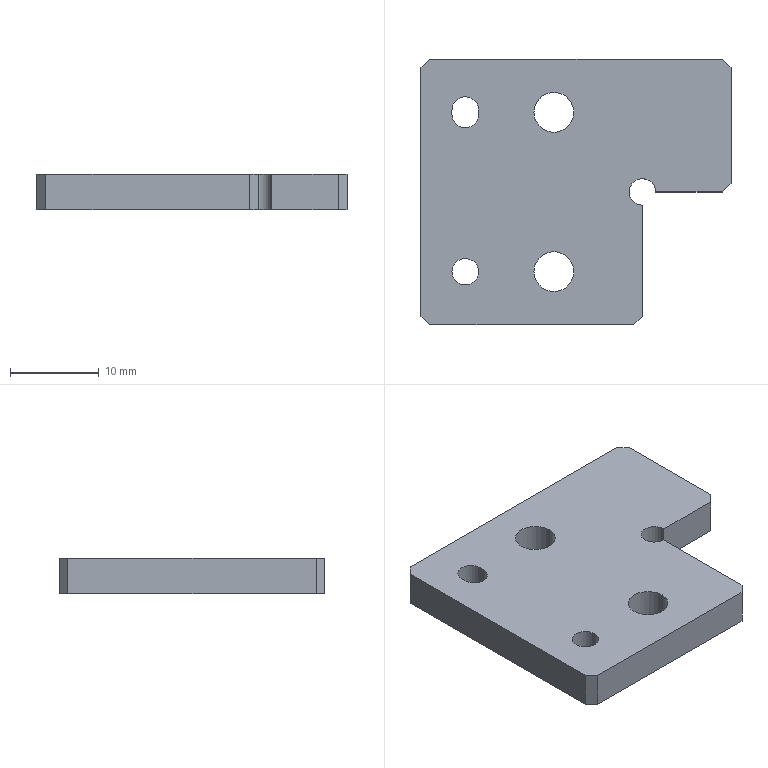Part | SolidWorks | features HoleWzd 3, ICE 2, Chamfer 1, Extrusion 1 | 1 solid | 24 faces | box 35 x 30 x 4 mm | volume 3379 mm3 | plane 15 | cylinder 9 | commonest cylinder face diameters 3 x5 4.5 x4
STEP:
#1=CARTESIAN_POINT('',(-4.75,9.,-2.));
#2=VERTEX_POINT('',#1);
#3=CARTESIAN_POINT('',(-0.25,9.,-2.));
#4=VERTEX_POINT('',#3);
#5=CARTESIAN_POINT('',(-2.5,9.,-2.));
#6=DIRECTION('',(0.,0.,1.));
#7=DIRECTION('',(1.,0.,0.));
#8=AXIS2_PLACEMENT_3D('',#5,#6,#7);
#9=CIRCLE('',#8,2.25);
#10=EDGE_CURVE('',#2,#4,#9,.T.);
#11=ORIENTED_EDGE('',*,*,#10,.F.);
#12=CARTESIAN_POINT('',(-4.75,9.,2.));
#13=VERTEX_POINT('',#12);
#14=CARTESIAN_POINT('',(-4.75,9.,2.));
#15=DIRECTION('',(0.,0.,1.));
#16=VECTOR('',#15,1000.);
#17=LINE('',#14,#16);
#18=EDGE_CURVE('',#2,#13,#17,.T.);
#19=ORIENTED_EDGE('',*,*,#18,.T.);
#20=CARTESIAN_POINT('',(-0.25,9.,2.));
#21=VERTEX_POINT('',#20);
#22=CARTESIAN_POINT('',(-2.5,9.,2.));
#23=DIRECTION('',(0.,0.,1.));
#24=DIRECTION('',(1.,0.,0.));
#25=AXIS2_PLACEMENT_3D('',#22,#23,#24);
#26=CIRCLE('',#25,2.25);
#27=EDGE_CURVE('',#13,#21,#26,.T.);
#28=ORIENTED_EDGE('',*,*,#27,.T.);
#29=CARTESIAN_POINT('',(-0.25,9.,2.));
#30=DIRECTION('',(0.,0.,1.));
#31=VECTOR('',#30,1000.);
#32=LINE('',#29,#31);
#33=EDGE_CURVE('',#4,#21,#32,.T.);
#34=ORIENTED_EDGE('',*,*,#33,.F.);
#35=EDGE_LOOP('',(#11,#19,#28,#34));
#36=FACE_OUTER_BOUND('',#35,.T.);
#37=CARTESIAN_POINT('',(-2.5,9.,2.));
#38=DIRECTION('',(0.,0.,1.));
#39=DIRECTION('',(1.,0.,0.));
#40=AXIS2_PLACEMENT_3D('',#37,#38,#39);
#41=CYLINDRICAL_SURFACE('',#40,2.25);
#42=ADVANCED_FACE('',(#36),#41,.F.);
#43=CARTESIAN_POINT('',(-4.75,-9.,-2.));
#44=VERTEX_POINT('',#43);
#45=CARTESIAN_POINT('',(-0.25,-9.,-2.));
#46=VERTEX_POINT('',#45);
#47=CARTESIAN_POINT('',(-2.5,-9.,-2.));
#48=DIRECTION('',(0.,0.,1.));
#49=DIRECTION('',(1.,0.,0.));
#50=AXIS2_PLACEMENT_3D('',#47,#48,#49);
#51=CIRCLE('',#50,2.25);
#52=EDGE_CURVE('',#44,#46,#51,.T.);
#53=ORIENTED_EDGE('',*,*,#52,.F.);
#54=CARTESIAN_POINT('',(-4.75,-9.,2.));
#55=VERTEX_POINT('',#54);
#56=CARTESIAN_POINT('',(-4.75,-9.,2.));
#57=DIRECTION('',(0.,0.,1.));
#58=VECTOR('',#57,1000.);
#59=LINE('',#56,#58);
#60=EDGE_CURVE('',#44,#55,#59,.T.);
#61=ORIENTED_EDGE('',*,*,#60,.T.);
#62=CARTESIAN_POINT('',(-0.25,-9.,2.));
#63=VERTEX_POINT('',#62);
#64=CARTESIAN_POINT('',(-2.5,-9.,2.));
#65=DIRECTION('',(0.,0.,1.));
#66=DIRECTION('',(1.,0.,0.));
#67=AXIS2_PLACEMENT_3D('',#64,#65,#66);
#68=CIRCLE('',#67,2.25);
#69=EDGE_CURVE('',#55,#63,#68,.T.);
#70=ORIENTED_EDGE('',*,*,#69,.T.);
#71=CARTESIAN_POINT('',(-0.25,-9.,2.));
#72=DIRECTION('',(0.,0.,1.));
#73=VECTOR('',#72,1000.);
#74=LINE('',#71,#73);
#75=EDGE_CURVE('',#46,#63,#74,.T.);
#76=ORIENTED_EDGE('',*,*,#75,.F.);
#77=EDGE_LOOP('',(#53,#61,#70,#76));
#78=FACE_OUTER_BOUND('',#77,.T.);
#79=CARTESIAN_POINT('',(-2.5,-9.,2.));
#80=DIRECTION('',(0.,0.,1.));
#81=DIRECTION('',(1.,0.,0.));
#82=AXIS2_PLACEMENT_3D('',#79,#80,#81);
#83=CYLINDRICAL_SURFACE('',#82,2.25);
#84=ADVANCED_FACE('',(#78),#83,.F.);
#85=CARTESIAN_POINT('',(-14.,-9.,-2.));
#86=VERTEX_POINT('',#85);
#87=CARTESIAN_POINT('',(-11.,-9.,-2.));
#88=VERTEX_POINT('',#87);
#89=CARTESIAN_POINT('',(-12.5,-9.,-2.));
#90=DIRECTION('',(0.,0.,1.));
#91=DIRECTION('',(1.,0.,0.));
#92=AXIS2_PLACEMENT_3D('',#89,#90,#91);
#93=CIRCLE('',#92,1.5);
#94=EDGE_CURVE('',#86,#88,#93,.T.);
#95=ORIENTED_EDGE('',*,*,#94,.F.);
#96=CARTESIAN_POINT('',(-14.,-9.,2.));
#97=VERTEX_POINT('',#96);
#98=CARTESIAN_POINT('',(-14.,-9.,2.));
#99=DIRECTION('',(0.,0.,1.));
#100=VECTOR('',#99,1000.);
#101=LINE('',#98,#100);
#102=EDGE_CURVE('',#86,#97,#101,.T.);
#103=ORIENTED_EDGE('',*,*,#102,.T.);
#104=CARTESIAN_POINT('',(-11.,-9.,2.));
#105=VERTEX_POINT('',#104);
#106=CARTESIAN_POINT('',(-12.5,-9.,2.));
#107=DIRECTION('',(0.,0.,1.));
#108=DIRECTION('',(1.,0.,0.));
#109=AXIS2_PLACEMENT_3D('',#106,#107,#108);
#110=CIRCLE('',#109,1.5);
#111=EDGE_CURVE('',#97,#105,#110,.T.);
#112=ORIENTED_EDGE('',*,*,#111,.T.);
#113=CARTESIAN_POINT('',(-11.,-9.,2.));
#114=DIRECTION('',(0.,0.,1.));
#115=VECTOR('',#114,1000.);
#116=LINE('',#113,#115);
#117=EDGE_CURVE('',#88,#105,#116,.T.);
#118=ORIENTED_EDGE('',*,*,#117,.F.);
#119=EDGE_LOOP('',(#95,#103,#112,#118));
#120=FACE_OUTER_BOUND('',#119,.T.);
#121=CARTESIAN_POINT('',(-12.5,-9.,2.));
#122=DIRECTION('',(0.,0.,1.));
#123=DIRECTION('',(1.,0.,0.));
#124=AXIS2_PLACEMENT_3D('',#121,#122,#123);
#125=CYLINDRICAL_SURFACE('',#124,1.5);
#126=ADVANCED_FACE('',(#120),#125,.F.);
#127=CARTESIAN_POINT('',(17.5,1.,-2.));
#128=VERTEX_POINT('',#127);
#129=CARTESIAN_POINT('',(17.5,14.,-2.));
#130=VERTEX_POINT('',#129);
#131=CARTESIAN_POINT('',(17.5,15.,-2.));
#132=DIRECTION('',(0.,1.,0.));
#133=VECTOR('',#132,1000.);
#134=LINE('',#131,#133);
#135=EDGE_CURVE('',#128,#130,#134,.T.);
#136=ORIENTED_EDGE('',*,*,#135,.T.);
#137=CARTESIAN_POINT('',(17.5,14.,2.));
#138=VERTEX_POINT('',#137);
#139=CARTESIAN_POINT('',(17.5,14.,2.));
#140=DIRECTION('',(0.,0.,1.));
#141=VECTOR('',#140,1000.);
#142=LINE('',#139,#141);
#143=EDGE_CURVE('',#130,#138,#142,.T.);
#144=ORIENTED_EDGE('',*,*,#143,.T.);
#145=CARTESIAN_POINT('',(17.5,1.,2.));
#146=VERTEX_POINT('',#145);
#147=CARTESIAN_POINT('',(17.5,15.,2.));
#148=DIRECTION('',(0.,1.,0.));
#149=VECTOR('',#148,1000.);
#150=LINE('',#147,#149);
#151=EDGE_CURVE('',#146,#138,#150,.T.);
#152=ORIENTED_EDGE('',*,*,#151,.F.);
#153=CARTESIAN_POINT('',(17.5,1.,2.));
#154=DIRECTION('',(0.,0.,-1.));
#155=VECTOR('',#154,1000.);
#156=LINE('',#153,#155);
#157=EDGE_CURVE('',#146,#128,#156,.T.);
#158=ORIENTED_EDGE('',*,*,#157,.T.);
#159=EDGE_LOOP('',(#136,#144,#152,#158));
#160=FACE_OUTER_BOUND('',#159,.T.);
#161=CARTESIAN_POINT('',(17.5,15.,2.));
#162=DIRECTION('',(-1.,0.,0.));
#163=DIRECTION('',(0.,-1.,0.));
#164=AXIS2_PLACEMENT_3D('',#161,#162,#163);
#165=PLANE('',#164);
#166=ADVANCED_FACE('',(#160),#165,.F.);
#167=CARTESIAN_POINT('',(16.5,15.,-2.));
#168=VERTEX_POINT('',#167);
#169=CARTESIAN_POINT('',(-16.5,15.,-2.));
#170=VERTEX_POINT('',#169);
#171=CARTESIAN_POINT('',(-17.5,15.,-2.));
#172=DIRECTION('',(-1.,0.,0.));
#173=VECTOR('',#172,1000.);
#174=LINE('',#171,#173);
#175=EDGE_CURVE('',#168,#170,#174,.T.);
#176=ORIENTED_EDGE('',*,*,#175,.T.);
#177=CARTESIAN_POINT('',(-16.5,15.,2.));
#178=VERTEX_POINT('',#177);
#179=CARTESIAN_POINT('',(-16.5,15.,2.));
#180=DIRECTION('',(0.,0.,1.));
#181=VECTOR('',#180,1000.);
#182=LINE('',#179,#181);
#183=EDGE_CURVE('',#170,#178,#182,.T.);
#184=ORIENTED_EDGE('',*,*,#183,.T.);
#185=CARTESIAN_POINT('',(16.5,15.,2.));
#186=VERTEX_POINT('',#185);
#187=CARTESIAN_POINT('',(-17.5,15.,2.));
#188=DIRECTION('',(-1.,0.,0.));
#189=VECTOR('',#188,1000.);
#190=LINE('',#187,#189);
#191=EDGE_CURVE('',#186,#178,#190,.T.);
#192=ORIENTED_EDGE('',*,*,#191,.F.);
#193=CARTESIAN_POINT('',(16.5,15.,2.));
#194=DIRECTION('',(0.,0.,-1.));
#195=VECTOR('',#194,1000.);
#196=LINE('',#193,#195);
#197=EDGE_CURVE('',#186,#168,#196,.T.);
#198=ORIENTED_EDGE('',*,*,#197,.T.);
#199=EDGE_LOOP('',(#176,#184,#192,#198));
#200=FACE_OUTER_BOUND('',#199,.T.);
#201=CARTESIAN_POINT('',(-17.5,15.,2.));
#202=DIRECTION('',(0.,-1.,0.));
#203=DIRECTION('',(0.,0.,-1.));
#204=AXIS2_PLACEMENT_3D('',#201,#202,#203);
#205=PLANE('',#204);
#206=ADVANCED_FACE('',(#200),#205,.F.);
#207=CARTESIAN_POINT('',(-17.5,14.,2.));
#208=VERTEX_POINT('',#207);
#209=CARTESIAN_POINT('',(-17.5,-14.,2.));
#210=VERTEX_POINT('',#209);
#211=CARTESIAN_POINT('',(-17.5,15.,2.));
#212=DIRECTION('',(0.,-1.,0.));
#213=VECTOR('',#212,1000.);
#214=LINE('',#211,#213);
#215=EDGE_CURVE('',#208,#210,#214,.T.);
#216=ORIENTED_EDGE('',*,*,#215,.F.);
#217=CARTESIAN_POINT('',(-17.5,14.,-2.));
#218=VERTEX_POINT('',#217);
#219=CARTESIAN_POINT('',(-17.5,14.,2.));
#220=DIRECTION('',(0.,0.,-1.));
#221=VECTOR('',#220,1000.);
#222=LINE('',#219,#221);
#223=EDGE_CURVE('',#208,#218,#222,.T.);
#224=ORIENTED_EDGE('',*,*,#223,.T.);
#225=CARTESIAN_POINT('',(-17.5,-14.,-2.));
#226=VERTEX_POINT('',#225);
#227=CARTESIAN_POINT('',(-17.5,15.,-2.));
#228=DIRECTION('',(0.,-1.,0.));
#229=VECTOR('',#228,1000.);
#230=LINE('',#227,#229);
#231=EDGE_CURVE('',#218,#226,#230,.T.);
#232=ORIENTED_EDGE('',*,*,#231,.T.);
#233=CARTESIAN_POINT('',(-17.5,-14.,2.));
#234=DIRECTION('',(0.,0.,1.));
#235=VECTOR('',#234,1000.);
#236=LINE('',#233,#235);
#237=EDGE_CURVE('',#226,#210,#236,.T.);
#238=ORIENTED_EDGE('',*,*,#237,.T.);
#239=EDGE_LOOP('',(#216,#224,#232,#238));
#240=FACE_OUTER_BOUND('',#239,.T.);
#241=CARTESIAN_POINT('',(-17.5,15.,2.));
#242=DIRECTION('',(1.,0.,0.));
#243=DIRECTION('',(0.,0.,-1.));
#244=AXIS2_PLACEMENT_3D('',#241,#242,#243);
#245=PLANE('',#244);
#246=ADVANCED_FACE('',(#240),#245,.F.);
#247=CARTESIAN_POINT('',(-16.5,-15.,-2.));
#248=VERTEX_POINT('',#247);
#249=CARTESIAN_POINT('',(6.5,-15.,-2.));
#250=VERTEX_POINT('',#249);
#251=CARTESIAN_POINT('',(-17.5,-15.,-2.));
#252=DIRECTION('',(1.,0.,0.));
#253=VECTOR('',#252,1000.);
#254=LINE('',#251,#253);
#255=EDGE_CURVE('',#248,#250,#254,.T.);
#256=ORIENTED_EDGE('',*,*,#255,.T.);
#257=CARTESIAN_POINT('',(6.5,-15.,2.));
#258=VERTEX_POINT('',#257);
#259=CARTESIAN_POINT('',(6.5,-15.,2.));
#260=DIRECTION('',(0.,0.,1.));
#261=VECTOR('',#260,1000.);
#262=LINE('',#259,#261);
#263=EDGE_CURVE('',#250,#258,#262,.T.);
#264=ORIENTED_EDGE('',*,*,#263,.T.);
#265=CARTESIAN_POINT('',(-16.5,-15.,2.));
#266=VERTEX_POINT('',#265);
#267=CARTESIAN_POINT('',(-17.5,-15.,2.));
#268=DIRECTION('',(1.,0.,0.));
#269=VECTOR('',#268,1000.);
#270=LINE('',#267,#269);
#271=EDGE_CURVE('',#266,#258,#270,.T.);
#272=ORIENTED_EDGE('',*,*,#271,.F.);
#273=CARTESIAN_POINT('',(-16.5,-15.,2.));
#274=DIRECTION('',(0.,0.,-1.));
#275=VECTOR('',#274,1000.);
#276=LINE('',#273,#275);
#277=EDGE_CURVE('',#266,#248,#276,.T.);
#278=ORIENTED_EDGE('',*,*,#277,.T.);
#279=EDGE_LOOP('',(#256,#264,#272,#278));
#280=FACE_OUTER_BOUND('',#279,.T.);
#281=CARTESIAN_POINT('',(-17.5,-15.,2.));
#282=DIRECTION('',(0.,1.,0.));
#283=DIRECTION('',(0.,0.,1.));
#284=AXIS2_PLACEMENT_3D('',#281,#282,#283);
#285=PLANE('',#284);
#286=ADVANCED_FACE('',(#280),#285,.F.);
#287=CARTESIAN_POINT('',(-11.,9.25,2.));
#288=VERTEX_POINT('',#287);
#289=CARTESIAN_POINT('',(-14.,9.25,2.));
#290=VERTEX_POINT('',#289);
#291=CARTESIAN_POINT('',(-12.5,9.25,2.));
#292=DIRECTION('',(0.,0.,1.));
#293=DIRECTION('',(1.,0.,0.));
#294=AXIS2_PLACEMENT_3D('',#291,#292,#293);
#295=CIRCLE('',#294,1.5);
#296=EDGE_CURVE('',#288,#290,#295,.T.);
#297=ORIENTED_EDGE('',*,*,#296,.F.);
#298=CARTESIAN_POINT('',(-11.,8.75,2.));
#299=VERTEX_POINT('',#298);
#300=CARTESIAN_POINT('',(-11.,9.25,2.));
#301=DIRECTION('',(0.,1.,0.));
#302=VECTOR('',#301,1000.);
#303=LINE('',#300,#302);
#304=EDGE_CURVE('',#299,#288,#303,.T.);
#305=ORIENTED_EDGE('',*,*,#304,.F.);
#306=CARTESIAN_POINT('',(-14.,8.75,2.));
#307=VERTEX_POINT('',#306);
#308=CARTESIAN_POINT('',(-12.5,8.75,2.));
#309=DIRECTION('',(0.,0.,1.));
#310=DIRECTION('',(1.,0.,0.));
#311=AXIS2_PLACEMENT_3D('',#308,#309,#310);
#312=CIRCLE('',#311,1.5);
#313=EDGE_CURVE('',#307,#299,#312,.T.);
#314=ORIENTED_EDGE('',*,*,#313,.F.);
#315=CARTESIAN_POINT('',(-14.,9.25,2.));
#316=DIRECTION('',(0.,-1.,0.));
#317=VECTOR('',#316,1000.);
#318=LINE('',#315,#317);
#319=EDGE_CURVE('',#290,#307,#318,.T.);
#320=ORIENTED_EDGE('',*,*,#319,.F.);
#321=EDGE_LOOP('',(#297,#305,#314,#320));
#322=FACE_BOUND('',#321,.T.);
#323=CARTESIAN_POINT('',(-2.5,9.,2.));
#324=DIRECTION('',(0.,0.,1.));
#325=DIRECTION('',(1.,0.,0.));
#326=AXIS2_PLACEMENT_3D('',#323,#324,#325);
#327=CIRCLE('',#326,2.25);
#328=EDGE_CURVE('',#21,#13,#327,.T.);
#329=ORIENTED_EDGE('',*,*,#328,.F.);
#330=ORIENTED_EDGE('',*,*,#27,.F.);
#331=EDGE_LOOP('',(#329,#330));
#332=FACE_BOUND('',#331,.T.);
#333=CARTESIAN_POINT('',(-2.5,-9.,2.));
#334=DIRECTION('',(0.,0.,1.));
#335=DIRECTION('',(1.,0.,0.));
#336=AXIS2_PLACEMENT_3D('',#333,#334,#335);
#337=CIRCLE('',#336,2.25);
#338=EDGE_CURVE('',#63,#55,#337,.T.);
#339=ORIENTED_EDGE('',*,*,#338,.F.);
#340=ORIENTED_EDGE('',*,*,#69,.F.);
#341=EDGE_LOOP('',(#339,#340));
#342=FACE_BOUND('',#341,.T.);
#343=CARTESIAN_POINT('',(-12.5,-9.,2.));
#344=DIRECTION('',(0.,0.,1.));
#345=DIRECTION('',(1.,0.,0.));
#346=AXIS2_PLACEMENT_3D('',#343,#344,#345);
#347=CIRCLE('',#346,1.5);
#348=EDGE_CURVE('',#105,#97,#347,.T.);
#349=ORIENTED_EDGE('',*,*,#348,.F.);
#350=ORIENTED_EDGE('',*,*,#111,.F.);
#351=EDGE_LOOP('',(#349,#350));
#352=FACE_BOUND('',#351,.T.);
#353=ORIENTED_EDGE('',*,*,#191,.T.);
#354=CARTESIAN_POINT('',(-15.75,15.75,2.));
#355=DIRECTION('',(-0.7071,-0.7071,0.));
#356=VECTOR('',#355,1000.);
#357=LINE('',#354,#356);
#358=EDGE_CURVE('',#178,#208,#357,.T.);
#359=ORIENTED_EDGE('',*,*,#358,.T.);
#360=ORIENTED_EDGE('',*,*,#215,.T.);
#361=CARTESIAN_POINT('',(-15.75,-15.75,2.));
#362=DIRECTION('',(0.7071,-0.7071,0.));
#363=VECTOR('',#362,1000.);
#364=LINE('',#361,#363);
#365=EDGE_CURVE('',#210,#266,#364,.T.);
#366=ORIENTED_EDGE('',*,*,#365,.T.);
#367=ORIENTED_EDGE('',*,*,#271,.T.);
#368=CARTESIAN_POINT('',(7.5,-14.,2.));
#369=VERTEX_POINT('',#368);
#370=CARTESIAN_POINT('',(10.75,-10.75,2.));
#371=DIRECTION('',(0.7071,0.7071,0.));
#372=VECTOR('',#371,1000.);
#373=LINE('',#370,#372);
#374=EDGE_CURVE('',#258,#369,#373,.T.);
#375=ORIENTED_EDGE('',*,*,#374,.T.);
#376=CARTESIAN_POINT('',(7.5,-1.5,2.));
#377=VERTEX_POINT('',#376);
#378=CARTESIAN_POINT('',(7.5,-15.,2.));
#379=DIRECTION('',(0.,-1.,0.));
#380=VECTOR('',#379,1000.);
#381=LINE('',#378,#380);
#382=EDGE_CURVE('',#377,#369,#381,.T.);
#383=ORIENTED_EDGE('',*,*,#382,.F.);
#384=CARTESIAN_POINT('',(9.,0.,2.));
#385=VERTEX_POINT('',#384);
#386=CARTESIAN_POINT('',(7.5,0.,2.));
#387=DIRECTION('',(0.,0.,1.));
#388=DIRECTION('',(1.,0.,0.));
#389=AXIS2_PLACEMENT_3D('',#386,#387,#388);
#390=CIRCLE('',#389,1.5);
#391=EDGE_CURVE('',#385,#377,#390,.T.);
#392=ORIENTED_EDGE('',*,*,#391,.F.);
#393=CARTESIAN_POINT('',(16.5,0.,2.));
#394=VERTEX_POINT('',#393);
#395=CARTESIAN_POINT('',(17.5,0.,2.));
#396=DIRECTION('',(-1.,0.,0.));
#397=VECTOR('',#396,1000.);
#398=LINE('',#395,#397);
#399=EDGE_CURVE('',#394,#385,#398,.T.);
#400=ORIENTED_EDGE('',*,*,#399,.F.);
#401=CARTESIAN_POINT('',(8.25,-8.25,2.));
#402=DIRECTION('',(0.7071,0.7071,0.));
#403=VECTOR('',#402,1000.);
#404=LINE('',#401,#403);
#405=EDGE_CURVE('',#394,#146,#404,.T.);
#406=ORIENTED_EDGE('',*,*,#405,.T.);
#407=ORIENTED_EDGE('',*,*,#151,.T.);
#408=CARTESIAN_POINT('',(15.75,15.75,2.));
#409=DIRECTION('',(-0.7071,0.7071,0.));
#410=VECTOR('',#409,1000.);
#411=LINE('',#408,#410);
#412=EDGE_CURVE('',#138,#186,#411,.T.);
#413=ORIENTED_EDGE('',*,*,#412,.T.);
#414=EDGE_LOOP('',(#353,#359,#360,#366,#367,#375,#383,#392,#400,#406,#407,#413));
#415=FACE_OUTER_BOUND('',#414,.T.);
#416=CARTESIAN_POINT('',(0.,0.,2.));
#417=DIRECTION('',(0.,0.,1.));
#418=DIRECTION('',(1.,0.,0.));
#419=AXIS2_PLACEMENT_3D('',#416,#417,#418);
#420=PLANE('',#419);
#421=ADVANCED_FACE('',(#322,#332,#342,#352,#415),#420,.T.);
#422=CARTESIAN_POINT('',(-2.5,9.,-2.));
#423=DIRECTION('',(0.,0.,1.));
#424=DIRECTION('',(1.,0.,0.));
#425=AXIS2_PLACEMENT_3D('',#422,#423,#424);
#426=CIRCLE('',#425,2.25);
#427=EDGE_CURVE('',#4,#2,#426,.T.);
#428=ORIENTED_EDGE('',*,*,#427,.T.);
#429=ORIENTED_EDGE('',*,*,#10,.T.);
#430=EDGE_LOOP('',(#428,#429));
#431=FACE_BOUND('',#430,.T.);
#432=CARTESIAN_POINT('',(-2.5,-9.,-2.));
#433=DIRECTION('',(0.,0.,1.));
#434=DIRECTION('',(1.,0.,0.));
#435=AXIS2_PLACEMENT_3D('',#432,#433,#434);
#436=CIRCLE('',#435,2.25);
#437=EDGE_CURVE('',#46,#44,#436,.T.);
#438=ORIENTED_EDGE('',*,*,#437,.T.);
#439=ORIENTED_EDGE('',*,*,#52,.T.);
#440=EDGE_LOOP('',(#438,#439));
#441=FACE_BOUND('',#440,.T.);
#442=CARTESIAN_POINT('',(-14.,8.75,-2.));
#443=VERTEX_POINT('',#442);
#444=CARTESIAN_POINT('',(-11.,8.75,-2.));
#445=VERTEX_POINT('',#444);
#446=CARTESIAN_POINT('',(-12.5,8.75,-2.));
#447=DIRECTION('',(0.,0.,1.));
#448=DIRECTION('',(1.,0.,0.));
#449=AXIS2_PLACEMENT_3D('',#446,#447,#448);
#450=CIRCLE('',#449,1.5);
#451=EDGE_CURVE('',#443,#445,#450,.T.);
#452=ORIENTED_EDGE('',*,*,#451,.T.);
#453=CARTESIAN_POINT('',(-11.,9.25,-2.));
#454=VERTEX_POINT('',#453);
#455=CARTESIAN_POINT('',(-11.,9.25,-2.));
#456=DIRECTION('',(0.,1.,0.));
#457=VECTOR('',#456,1000.);
#458=LINE('',#455,#457);
#459=EDGE_CURVE('',#445,#454,#458,.T.);
#460=ORIENTED_EDGE('',*,*,#459,.T.);
#461=CARTESIAN_POINT('',(-14.,9.25,-2.));
#462=VERTEX_POINT('',#461);
#463=CARTESIAN_POINT('',(-12.5,9.25,-2.));
#464=DIRECTION('',(0.,0.,1.));
#465=DIRECTION('',(1.,0.,0.));
#466=AXIS2_PLACEMENT_3D('',#463,#464,#465);
#467=CIRCLE('',#466,1.5);
#468=EDGE_CURVE('',#454,#462,#467,.T.);
#469=ORIENTED_EDGE('',*,*,#468,.T.);
#470=CARTESIAN_POINT('',(-14.,9.25,-2.));
#471=DIRECTION('',(0.,-1.,0.));
#472=VECTOR('',#471,1000.);
#473=LINE('',#470,#472);
#474=EDGE_CURVE('',#462,#443,#473,.T.);
#475=ORIENTED_EDGE('',*,*,#474,.T.);
#476=EDGE_LOOP('',(#452,#460,#469,#475));
#477=FACE_BOUND('',#476,.T.);
#478=CARTESIAN_POINT('',(-12.5,-9.,-2.));
#479=DIRECTION('',(0.,0.,1.));
#480=DIRECTION('',(1.,0.,0.));
#481=AXIS2_PLACEMENT_3D('',#478,#479,#480);
#482=CIRCLE('',#481,1.5);
#483=EDGE_CURVE('',#88,#86,#482,.T.);
#484=ORIENTED_EDGE('',*,*,#483,.T.);
#485=ORIENTED_EDGE('',*,*,#94,.T.);
#486=EDGE_LOOP('',(#484,#485));
#487=FACE_BOUND('',#486,.T.);
#488=ORIENTED_EDGE('',*,*,#231,.F.);
#489=CARTESIAN_POINT('',(-17.5,14.,-2.));
#490=DIRECTION('',(0.7071,0.7071,0.));
#491=VECTOR('',#490,1000.);
#492=LINE('',#489,#491);
#493=EDGE_CURVE('',#218,#170,#492,.T.);
#494=ORIENTED_EDGE('',*,*,#493,.T.);
#495=ORIENTED_EDGE('',*,*,#175,.F.);
#496=CARTESIAN_POINT('',(16.5,15.,-2.));
#497=DIRECTION('',(0.7071,-0.7071,0.));
#498=VECTOR('',#497,1000.);
#499=LINE('',#496,#498);
#500=EDGE_CURVE('',#168,#130,#499,.T.);
#501=ORIENTED_EDGE('',*,*,#500,.T.);
#502=ORIENTED_EDGE('',*,*,#135,.F.);
#503=CARTESIAN_POINT('',(16.5,0.,-2.));
#504=VERTEX_POINT('',#503);
#505=CARTESIAN_POINT('',(16.5,0.,-2.));
#506=DIRECTION('',(-0.7071,-0.7071,0.));
#507=VECTOR('',#506,1000.);
#508=LINE('',#505,#507);
#509=EDGE_CURVE('',#128,#504,#508,.T.);
#510=ORIENTED_EDGE('',*,*,#509,.T.);
#511=CARTESIAN_POINT('',(9.,0.,-2.));
#512=VERTEX_POINT('',#511);
#513=CARTESIAN_POINT('',(17.5,0.,-2.));
#514=DIRECTION('',(-1.,0.,0.));
#515=VECTOR('',#514,1000.);
#516=LINE('',#513,#515);
#517=EDGE_CURVE('',#504,#512,#516,.T.);
#518=ORIENTED_EDGE('',*,*,#517,.T.);
#519=CARTESIAN_POINT('',(7.5,-1.5,-2.));
#520=VERTEX_POINT('',#519);
#521=CARTESIAN_POINT('',(7.5,0.,-2.));
#522=DIRECTION('',(0.,0.,1.));
#523=DIRECTION('',(1.,0.,0.));
#524=AXIS2_PLACEMENT_3D('',#521,#522,#523);
#525=CIRCLE('',#524,1.5);
#526=EDGE_CURVE('',#512,#520,#525,.T.);
#527=ORIENTED_EDGE('',*,*,#526,.T.);
#528=CARTESIAN_POINT('',(7.5,-14.,-2.));
#529=VERTEX_POINT('',#528);
#530=CARTESIAN_POINT('',(7.5,-15.,-2.));
#531=DIRECTION('',(0.,-1.,0.));
#532=VECTOR('',#531,1000.);
#533=LINE('',#530,#532);
#534=EDGE_CURVE('',#520,#529,#533,.T.);
#535=ORIENTED_EDGE('',*,*,#534,.T.);
#536=CARTESIAN_POINT('',(6.5,-15.,-2.));
#537=DIRECTION('',(-0.7071,-0.7071,0.));
#538=VECTOR('',#537,1000.);
#539=LINE('',#536,#538);
#540=EDGE_CURVE('',#529,#250,#539,.T.);
#541=ORIENTED_EDGE('',*,*,#540,.T.);
#542=ORIENTED_EDGE('',*,*,#255,.F.);
#543=CARTESIAN_POINT('',(-16.5,-15.,-2.));
#544=DIRECTION('',(-0.7071,0.7071,0.));
#545=VECTOR('',#544,1000.);
#546=LINE('',#543,#545);
#547=EDGE_CURVE('',#248,#226,#546,.T.);
#548=ORIENTED_EDGE('',*,*,#547,.T.);
#549=EDGE_LOOP('',(#488,#494,#495,#501,#502,#510,#518,#527,#535,#541,#542,#548));
#550=FACE_OUTER_BOUND('',#549,.T.);
#551=CARTESIAN_POINT('',(0.,0.,-2.));
#552=DIRECTION('',(0.,0.,1.));
#553=DIRECTION('',(1.,0.,0.));
#554=AXIS2_PLACEMENT_3D('',#551,#552,#553);
#555=PLANE('',#554);
#556=ADVANCED_FACE('',(#431,#441,#477,#487,#550),#555,.F.);
#557=ORIENTED_EDGE('',*,*,#382,.T.);
#558=CARTESIAN_POINT('',(7.5,-14.,-2.));
#559=DIRECTION('',(0.,0.,-1.));
#560=VECTOR('',#559,1000.);
#561=LINE('',#558,#560);
#562=EDGE_CURVE('',#369,#529,#561,.T.);
#563=ORIENTED_EDGE('',*,*,#562,.T.);
#564=ORIENTED_EDGE('',*,*,#534,.F.);
#565=CARTESIAN_POINT('',(7.5,-1.5,2.));
#566=DIRECTION('',(0.,0.,1.));
#567=VECTOR('',#566,1000.);
#568=LINE('',#565,#567);
#569=EDGE_CURVE('',#520,#377,#568,.T.);
#570=ORIENTED_EDGE('',*,*,#569,.T.);
#571=EDGE_LOOP('',(#557,#563,#564,#570));
#572=FACE_OUTER_BOUND('',#571,.T.);
#573=CARTESIAN_POINT('',(7.5,-15.,-2.));
#574=DIRECTION('',(-1.,0.,0.));
#575=DIRECTION('',(0.,0.,1.));
#576=AXIS2_PLACEMENT_3D('',#573,#574,#575);
#577=PLANE('',#576);
#578=ADVANCED_FACE('',(#572),#577,.F.);
#579=ORIENTED_EDGE('',*,*,#517,.F.);
#580=CARTESIAN_POINT('',(16.5,0.,-2.));
#581=DIRECTION('',(0.,0.,1.));
#582=VECTOR('',#581,1000.);
#583=LINE('',#580,#582);
#584=EDGE_CURVE('',#504,#394,#583,.T.);
#585=ORIENTED_EDGE('',*,*,#584,.T.);
#586=ORIENTED_EDGE('',*,*,#399,.T.);
#587=CARTESIAN_POINT('',(9.,0.,2.));
#588=DIRECTION('',(0.,0.,-1.));
#589=VECTOR('',#588,1000.);
#590=LINE('',#587,#589);
#591=EDGE_CURVE('',#385,#512,#590,.T.);
#592=ORIENTED_EDGE('',*,*,#591,.T.);
#593=EDGE_LOOP('',(#579,#585,#586,#592));
#594=FACE_OUTER_BOUND('',#593,.T.);
#595=CARTESIAN_POINT('',(17.5,0.,-2.));
#596=DIRECTION('',(0.,1.,0.));
#597=DIRECTION('',(-1.,0.,0.));
#598=AXIS2_PLACEMENT_3D('',#595,#596,#597);
#599=PLANE('',#598);
#600=ADVANCED_FACE('',(#594),#599,.F.);
#601=ORIENTED_EDGE('',*,*,#526,.F.);
#602=ORIENTED_EDGE('',*,*,#591,.F.);
#603=ORIENTED_EDGE('',*,*,#391,.T.);
#604=ORIENTED_EDGE('',*,*,#569,.F.);
#605=EDGE_LOOP('',(#601,#602,#603,#604));
#606=FACE_OUTER_BOUND('',#605,.T.);
#607=CARTESIAN_POINT('',(7.5,0.,2.));
#608=DIRECTION('',(0.,0.,1.));
#609=DIRECTION('',(1.,0.,0.));
#610=AXIS2_PLACEMENT_3D('',#607,#608,#609);
#611=CYLINDRICAL_SURFACE('',#610,1.5);
#612=ADVANCED_FACE('',(#606),#611,.F.);
#613=ORIENTED_EDGE('',*,*,#102,.F.);
#614=ORIENTED_EDGE('',*,*,#483,.F.);
#615=ORIENTED_EDGE('',*,*,#117,.T.);
#616=ORIENTED_EDGE('',*,*,#348,.T.);
#617=EDGE_LOOP('',(#613,#614,#615,#616));
#618=FACE_OUTER_BOUND('',#617,.T.);
#619=CARTESIAN_POINT('',(-12.5,-9.,2.));
#620=DIRECTION('',(0.,0.,1.));
#621=DIRECTION('',(1.,0.,0.));
#622=AXIS2_PLACEMENT_3D('',#619,#620,#621);
#623=CYLINDRICAL_SURFACE('',#622,1.5);
#624=ADVANCED_FACE('',(#618),#623,.F.);
#625=ORIENTED_EDGE('',*,*,#60,.F.);
#626=ORIENTED_EDGE('',*,*,#437,.F.);
#627=ORIENTED_EDGE('',*,*,#75,.T.);
#628=ORIENTED_EDGE('',*,*,#338,.T.);
#629=EDGE_LOOP('',(#625,#626,#627,#628));
#630=FACE_OUTER_BOUND('',#629,.T.);
#631=CARTESIAN_POINT('',(-2.5,-9.,2.));
#632=DIRECTION('',(0.,0.,1.));
#633=DIRECTION('',(1.,0.,0.));
#634=AXIS2_PLACEMENT_3D('',#631,#632,#633);
#635=CYLINDRICAL_SURFACE('',#634,2.25);
#636=ADVANCED_FACE('',(#630),#635,.F.);
#637=ORIENTED_EDGE('',*,*,#18,.F.);
#638=ORIENTED_EDGE('',*,*,#427,.F.);
#639=ORIENTED_EDGE('',*,*,#33,.T.);
#640=ORIENTED_EDGE('',*,*,#328,.T.);
#641=EDGE_LOOP('',(#637,#638,#639,#640));
#642=FACE_OUTER_BOUND('',#641,.T.);
#643=CARTESIAN_POINT('',(-2.5,9.,2.));
#644=DIRECTION('',(0.,0.,1.));
#645=DIRECTION('',(1.,0.,0.));
#646=AXIS2_PLACEMENT_3D('',#643,#644,#645);
#647=CYLINDRICAL_SURFACE('',#646,2.25);
#648=ADVANCED_FACE('',(#642),#647,.F.);
#649=ORIENTED_EDGE('',*,*,#358,.F.);
#650=ORIENTED_EDGE('',*,*,#183,.F.);
#651=ORIENTED_EDGE('',*,*,#493,.F.);
#652=ORIENTED_EDGE('',*,*,#223,.F.);
#653=EDGE_LOOP('',(#649,#650,#651,#652));
#654=FACE_OUTER_BOUND('',#653,.T.);
#655=CARTESIAN_POINT('',(-17.5,14.,2.));
#656=DIRECTION('',(0.7071,-0.7071,0.));
#657=DIRECTION('',(0.,0.,-1.));
#658=AXIS2_PLACEMENT_3D('',#655,#656,#657);
#659=PLANE('',#658);
#660=ADVANCED_FACE('',(#654),#659,.F.);
#661=ORIENTED_EDGE('',*,*,#412,.F.);
#662=ORIENTED_EDGE('',*,*,#143,.F.);
#663=ORIENTED_EDGE('',*,*,#500,.F.);
#664=ORIENTED_EDGE('',*,*,#197,.F.);
#665=EDGE_LOOP('',(#661,#662,#663,#664));
#666=FACE_OUTER_BOUND('',#665,.T.);
#667=CARTESIAN_POINT('',(16.5,15.,2.));
#668=DIRECTION('',(-0.7071,-0.7071,0.));
#669=DIRECTION('',(0.,0.,-1.));
#670=AXIS2_PLACEMENT_3D('',#667,#668,#669);
#671=PLANE('',#670);
#672=ADVANCED_FACE('',(#666),#671,.F.);
#673=ORIENTED_EDGE('',*,*,#509,.F.);
#674=ORIENTED_EDGE('',*,*,#157,.F.);
#675=ORIENTED_EDGE('',*,*,#405,.F.);
#676=ORIENTED_EDGE('',*,*,#584,.F.);
#677=EDGE_LOOP('',(#673,#674,#675,#676));
#678=FACE_OUTER_BOUND('',#677,.T.);
#679=CARTESIAN_POINT('',(16.5,0.,-2.));
#680=DIRECTION('',(-0.7071,0.7071,0.));
#681=DIRECTION('',(0.,0.,1.));
#682=AXIS2_PLACEMENT_3D('',#679,#680,#681);
#683=PLANE('',#682);
#684=ADVANCED_FACE('',(#678),#683,.F.);
#685=ORIENTED_EDGE('',*,*,#540,.F.);
#686=ORIENTED_EDGE('',*,*,#562,.F.);
#687=ORIENTED_EDGE('',*,*,#374,.F.);
#688=ORIENTED_EDGE('',*,*,#263,.F.);
#689=EDGE_LOOP('',(#685,#686,#687,#688));
#690=FACE_OUTER_BOUND('',#689,.T.);
#691=CARTESIAN_POINT('',(6.5,-15.,2.));
#692=DIRECTION('',(-0.7071,0.7071,0.));
#693=DIRECTION('',(0.,0.,1.));
#694=AXIS2_PLACEMENT_3D('',#691,#692,#693);
#695=PLANE('',#694);
#696=ADVANCED_FACE('',(#690),#695,.F.);
#697=ORIENTED_EDGE('',*,*,#365,.F.);
#698=ORIENTED_EDGE('',*,*,#237,.F.);
#699=ORIENTED_EDGE('',*,*,#547,.F.);
#700=ORIENTED_EDGE('',*,*,#277,.F.);
#701=EDGE_LOOP('',(#697,#698,#699,#700));
#702=FACE_OUTER_BOUND('',#701,.T.);
#703=CARTESIAN_POINT('',(-16.5,-15.,2.));
#704=DIRECTION('',(0.7071,0.7071,0.));
#705=DIRECTION('',(0.,0.,-1.));
#706=AXIS2_PLACEMENT_3D('',#703,#704,#705);
#707=PLANE('',#706);
#708=ADVANCED_FACE('',(#702),#707,.F.);
#709=ORIENTED_EDGE('',*,*,#304,.T.);
#710=CARTESIAN_POINT('',(-11.,9.25,-2.));
#711=DIRECTION('',(0.,0.,1.));
#712=VECTOR('',#711,1000.);
#713=LINE('',#710,#712);
#714=EDGE_CURVE('',#454,#288,#713,.T.);
#715=ORIENTED_EDGE('',*,*,#714,.F.);
#716=ORIENTED_EDGE('',*,*,#459,.F.);
#717=CARTESIAN_POINT('',(-11.,8.75,-2.));
#718=DIRECTION('',(0.,0.,1.));
#719=VECTOR('',#718,1000.);
#720=LINE('',#717,#719);
#721=EDGE_CURVE('',#445,#299,#720,.T.);
#722=ORIENTED_EDGE('',*,*,#721,.T.);
#723=EDGE_LOOP('',(#709,#715,#716,#722));
#724=FACE_OUTER_BOUND('',#723,.T.);
#725=CARTESIAN_POINT('',(-11.,9.25,-2.));
#726=DIRECTION('',(1.,0.,0.));
#727=DIRECTION('',(0.,0.,-1.));
#728=AXIS2_PLACEMENT_3D('',#725,#726,#727);
#729=PLANE('',#728);
#730=ADVANCED_FACE('',(#724),#729,.F.);
#731=ORIENTED_EDGE('',*,*,#319,.T.);
#732=CARTESIAN_POINT('',(-14.,8.75,-2.));
#733=DIRECTION('',(0.,0.,1.));
#734=VECTOR('',#733,1000.);
#735=LINE('',#732,#734);
#736=EDGE_CURVE('',#443,#307,#735,.T.);
#737=ORIENTED_EDGE('',*,*,#736,.F.);
#738=ORIENTED_EDGE('',*,*,#474,.F.);
#739=CARTESIAN_POINT('',(-14.,9.25,-2.));
#740=DIRECTION('',(0.,0.,1.));
#741=VECTOR('',#740,1000.);
#742=LINE('',#739,#741);
#743=EDGE_CURVE('',#462,#290,#742,.T.);
#744=ORIENTED_EDGE('',*,*,#743,.T.);
#745=EDGE_LOOP('',(#731,#737,#738,#744));
#746=FACE_OUTER_BOUND('',#745,.T.);
#747=CARTESIAN_POINT('',(-14.,9.25,-2.));
#748=DIRECTION('',(-1.,0.,0.));
#749=DIRECTION('',(0.,0.,1.));
#750=AXIS2_PLACEMENT_3D('',#747,#748,#749);
#751=PLANE('',#750);
#752=ADVANCED_FACE('',(#746),#751,.F.);
#753=ORIENTED_EDGE('',*,*,#296,.T.);
#754=ORIENTED_EDGE('',*,*,#743,.F.);
#755=ORIENTED_EDGE('',*,*,#468,.F.);
#756=ORIENTED_EDGE('',*,*,#714,.T.);
#757=EDGE_LOOP('',(#753,#754,#755,#756));
#758=FACE_OUTER_BOUND('',#757,.T.);
#759=CARTESIAN_POINT('',(-12.5,9.25,-2.));
#760=DIRECTION('',(0.,0.,1.));
#761=DIRECTION('',(1.,0.,0.));
#762=AXIS2_PLACEMENT_3D('',#759,#760,#761);
#763=CYLINDRICAL_SURFACE('',#762,1.5);
#764=ADVANCED_FACE('',(#758),#763,.F.);
#765=ORIENTED_EDGE('',*,*,#313,.T.);
#766=ORIENTED_EDGE('',*,*,#721,.F.);
#767=ORIENTED_EDGE('',*,*,#451,.F.);
#768=ORIENTED_EDGE('',*,*,#736,.T.);
#769=EDGE_LOOP('',(#765,#766,#767,#768));
#770=FACE_OUTER_BOUND('',#769,.T.);
#771=CARTESIAN_POINT('',(-12.5,8.75,-2.));
#772=DIRECTION('',(0.,0.,1.));
#773=DIRECTION('',(1.,0.,0.));
#774=AXIS2_PLACEMENT_3D('',#771,#772,#773);
#775=CYLINDRICAL_SURFACE('',#774,1.5);
#776=ADVANCED_FACE('',(#770),#775,.F.);
#777=CLOSED_SHELL('',(#42,#84,#126,#166,#206,#246,#286,#421,#556,#578,#600,#612,#624,#636,#648,#660,#672,#684,#696,#708,#730,#752,#764,#776));
#778=MANIFOLD_SOLID_BREP('',#777);
#779=CARTESIAN_POINT('',(0.,0.,0.));
#780=DIRECTION('',(0.,0.,1.));
#781=DIRECTION('',(1.,0.,0.));
#782=AXIS2_PLACEMENT_3D('',#779,#780,#781);
#783=(LENGTH_UNIT()NAMED_UNIT(*)SI_UNIT(.MILLI.,.METRE.));
#784=UNCERTAINTY_MEASURE_WITH_UNIT(LENGTH_MEASURE(0.00001),#783,'','');
#785=(NAMED_UNIT(*)PLANE_ANGLE_UNIT()SI_UNIT($,.RADIAN.));
#786=(NAMED_UNIT(*)SI_UNIT($,.STERADIAN.)SOLID_ANGLE_UNIT());
#787=(GEOMETRIC_REPRESENTATION_CONTEXT(3)GLOBAL_UNCERTAINTY_ASSIGNED_CONTEXT((#784))GLOBAL_UNIT_ASSIGNED_CONTEXT((#783,#785,#786))REPRESENTATION_CONTEXT('',''));
#788=ADVANCED_BREP_SHAPE_REPRESENTATION('',(#778,#782),#787);